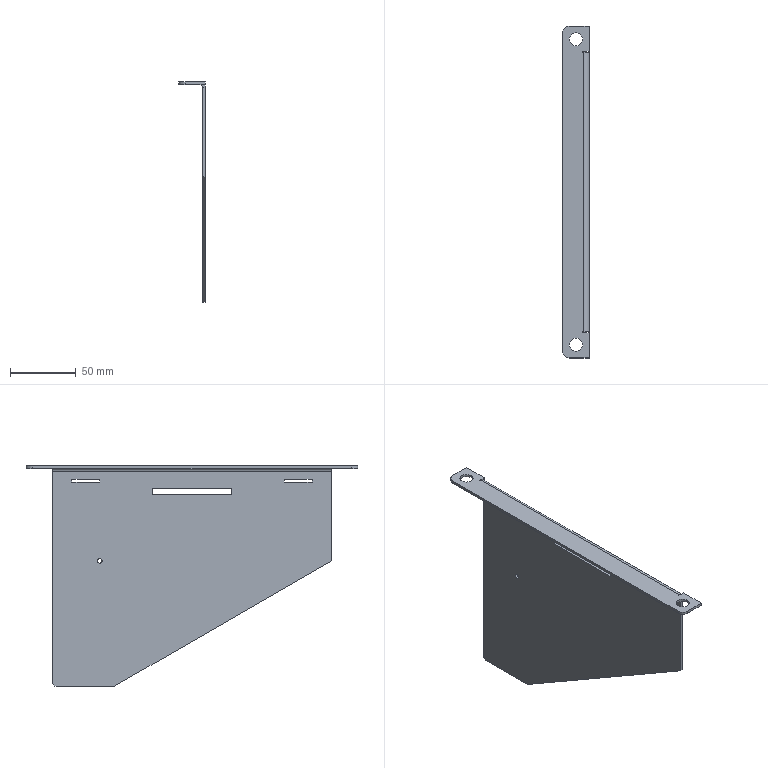Part | STEP file | SYL0380DJ1008_2_7_2_1-1_STEP | 1 solid | 44 faces | box 20 x 252 x 167 mm | volume 62697 mm3 | plane 34 | cylinder 10 | commonest cylinder face diameters 10 x6 3.5 x2 4 x1 8 x1
STEP:
#1=CARTESIAN_POINT('',(10.,-30.,-15.));
#2=VERTEX_POINT('',#1);
#3=CARTESIAN_POINT('',(8.,-30.,-15.));
#4=VERTEX_POINT('',#3);
#5=CARTESIAN_POINT('',(8.,-30.,-15.));
#6=DIRECTION('',(-1.,0.,0.));
#7=VECTOR('',#6,1000.);
#8=LINE('',#5,#7);
#9=EDGE_CURVE('',#2,#4,#8,.T.);
#10=ORIENTED_EDGE('',*,*,#9,.F.);
#11=CARTESIAN_POINT('',(10.,-30.,-20.));
#12=VERTEX_POINT('',#11);
#13=CARTESIAN_POINT('',(10.,-30.,2.));
#14=DIRECTION('',(0.,0.,-1.));
#15=VECTOR('',#14,1000.);
#16=LINE('',#13,#15);
#17=EDGE_CURVE('',#2,#12,#16,.T.);
#18=ORIENTED_EDGE('',*,*,#17,.T.);
#19=CARTESIAN_POINT('',(8.,-30.,-20.));
#20=VERTEX_POINT('',#19);
#21=CARTESIAN_POINT('',(8.,-30.,-20.));
#22=DIRECTION('',(-1.,0.,0.));
#23=VECTOR('',#22,1000.);
#24=LINE('',#21,#23);
#25=EDGE_CURVE('',#12,#20,#24,.T.);
#26=ORIENTED_EDGE('',*,*,#25,.T.);
#27=CARTESIAN_POINT('',(8.,-30.,-15.));
#28=DIRECTION('',(0.,0.,-1.));
#29=VECTOR('',#28,1000.);
#30=LINE('',#27,#29);
#31=EDGE_CURVE('',#4,#20,#30,.T.);
#32=ORIENTED_EDGE('',*,*,#31,.F.);
#33=EDGE_LOOP('',(#10,#18,#26,#32));
#34=FACE_OUTER_BOUND('',#33,.T.);
#35=CARTESIAN_POINT('',(8.,-30.,-15.));
#36=DIRECTION('',(0.,-1.,0.));
#37=DIRECTION('',(0.,0.,-1.));
#38=AXIS2_PLACEMENT_3D('',#35,#36,#37);
#39=PLANE('',#38);
#40=ADVANCED_FACE('',(#34),#39,.F.);
#41=ORIENTED_EDGE('',*,*,#25,.F.);
#42=CARTESIAN_POINT('',(10.,30.,-20.));
#43=VERTEX_POINT('',#42);
#44=CARTESIAN_POINT('',(10.,-66.125,-20.));
#45=DIRECTION('',(0.,1.,0.));
#46=VECTOR('',#45,1000.);
#47=LINE('',#44,#46);
#48=EDGE_CURVE('',#12,#43,#47,.T.);
#49=ORIENTED_EDGE('',*,*,#48,.T.);
#50=CARTESIAN_POINT('',(8.,30.,-20.));
#51=VERTEX_POINT('',#50);
#52=CARTESIAN_POINT('',(8.,30.,-20.));
#53=DIRECTION('',(-1.,0.,0.));
#54=VECTOR('',#53,1000.);
#55=LINE('',#52,#54);
#56=EDGE_CURVE('',#43,#51,#55,.T.);
#57=ORIENTED_EDGE('',*,*,#56,.T.);
#58=CARTESIAN_POINT('',(8.,-30.,-20.));
#59=DIRECTION('',(0.,1.,0.));
#60=VECTOR('',#59,1000.);
#61=LINE('',#58,#60);
#62=EDGE_CURVE('',#20,#51,#61,.T.);
#63=ORIENTED_EDGE('',*,*,#62,.F.);
#64=EDGE_LOOP('',(#41,#49,#57,#63));
#65=FACE_OUTER_BOUND('',#64,.T.);
#66=CARTESIAN_POINT('',(8.,-30.,-20.));
#67=DIRECTION('',(0.,0.,-1.));
#68=DIRECTION('',(0.,1.,0.));
#69=AXIS2_PLACEMENT_3D('',#66,#67,#68);
#70=PLANE('',#69);
#71=ADVANCED_FACE('',(#65),#70,.F.);
#72=ORIENTED_EDGE('',*,*,#56,.F.);
#73=CARTESIAN_POINT('',(10.,30.,-15.));
#74=VERTEX_POINT('',#73);
#75=CARTESIAN_POINT('',(10.,30.,2.));
#76=DIRECTION('',(0.,0.,1.));
#77=VECTOR('',#76,1000.);
#78=LINE('',#75,#77);
#79=EDGE_CURVE('',#43,#74,#78,.T.);
#80=ORIENTED_EDGE('',*,*,#79,.T.);
#81=CARTESIAN_POINT('',(8.,30.,-15.));
#82=VERTEX_POINT('',#81);
#83=CARTESIAN_POINT('',(8.,30.,-15.));
#84=DIRECTION('',(-1.,0.,0.));
#85=VECTOR('',#84,1000.);
#86=LINE('',#83,#85);
#87=EDGE_CURVE('',#74,#82,#86,.T.);
#88=ORIENTED_EDGE('',*,*,#87,.T.);
#89=CARTESIAN_POINT('',(8.,30.,-20.));
#90=DIRECTION('',(0.,0.,1.));
#91=VECTOR('',#90,1000.);
#92=LINE('',#89,#91);
#93=EDGE_CURVE('',#51,#82,#92,.T.);
#94=ORIENTED_EDGE('',*,*,#93,.F.);
#95=EDGE_LOOP('',(#72,#80,#88,#94));
#96=FACE_OUTER_BOUND('',#95,.T.);
#97=CARTESIAN_POINT('',(8.,30.,-20.));
#98=DIRECTION('',(0.,1.,0.));
#99=DIRECTION('',(0.,0.,1.));
#100=AXIS2_PLACEMENT_3D('',#97,#98,#99);
#101=PLANE('',#100);
#102=ADVANCED_FACE('',(#96),#101,.F.);
#103=CARTESIAN_POINT('',(10.,70.,-8.));
#104=VERTEX_POINT('',#103);
#105=CARTESIAN_POINT('',(8.,70.,-8.));
#106=VERTEX_POINT('',#105);
#107=CARTESIAN_POINT('',(8.,70.,-8.));
#108=DIRECTION('',(-1.,0.,0.));
#109=VECTOR('',#108,1000.);
#110=LINE('',#107,#109);
#111=EDGE_CURVE('',#104,#106,#110,.T.);
#112=ORIENTED_EDGE('',*,*,#111,.F.);
#113=CARTESIAN_POINT('',(10.,70.,-10.2));
#114=VERTEX_POINT('',#113);
#115=CARTESIAN_POINT('',(10.,70.,2.));
#116=DIRECTION('',(0.,0.,-1.));
#117=VECTOR('',#116,1000.);
#118=LINE('',#115,#117);
#119=EDGE_CURVE('',#104,#114,#118,.T.);
#120=ORIENTED_EDGE('',*,*,#119,.T.);
#121=CARTESIAN_POINT('',(8.,70.,-10.2));
#122=VERTEX_POINT('',#121);
#123=CARTESIAN_POINT('',(8.,70.,-10.2));
#124=DIRECTION('',(-1.,0.,0.));
#125=VECTOR('',#124,1000.);
#126=LINE('',#123,#125);
#127=EDGE_CURVE('',#114,#122,#126,.T.);
#128=ORIENTED_EDGE('',*,*,#127,.T.);
#129=CARTESIAN_POINT('',(8.,70.,-8.));
#130=DIRECTION('',(0.,0.,-1.));
#131=VECTOR('',#130,1000.);
#132=LINE('',#129,#131);
#133=EDGE_CURVE('',#106,#122,#132,.T.);
#134=ORIENTED_EDGE('',*,*,#133,.F.);
#135=EDGE_LOOP('',(#112,#120,#128,#134));
#136=FACE_OUTER_BOUND('',#135,.T.);
#137=CARTESIAN_POINT('',(8.,70.,-8.));
#138=DIRECTION('',(0.,-1.,0.));
#139=DIRECTION('',(0.,0.,-1.));
#140=AXIS2_PLACEMENT_3D('',#137,#138,#139);
#141=PLANE('',#140);
#142=ADVANCED_FACE('',(#136),#141,.F.);
#143=ORIENTED_EDGE('',*,*,#127,.F.);
#144=CARTESIAN_POINT('',(10.,91.2,-10.2));
#145=VERTEX_POINT('',#144);
#146=CARTESIAN_POINT('',(10.,-66.125,-10.2));
#147=DIRECTION('',(0.,1.,0.));
#148=VECTOR('',#147,1000.);
#149=LINE('',#146,#148);
#150=EDGE_CURVE('',#114,#145,#149,.T.);
#151=ORIENTED_EDGE('',*,*,#150,.T.);
#152=CARTESIAN_POINT('',(8.,91.2,-10.2));
#153=VERTEX_POINT('',#152);
#154=CARTESIAN_POINT('',(8.,91.2,-10.2));
#155=DIRECTION('',(-1.,0.,0.));
#156=VECTOR('',#155,1000.);
#157=LINE('',#154,#156);
#158=EDGE_CURVE('',#145,#153,#157,.T.);
#159=ORIENTED_EDGE('',*,*,#158,.T.);
#160=CARTESIAN_POINT('',(8.,70.,-10.2));
#161=DIRECTION('',(0.,1.,0.));
#162=VECTOR('',#161,1000.);
#163=LINE('',#160,#162);
#164=EDGE_CURVE('',#122,#153,#163,.T.);
#165=ORIENTED_EDGE('',*,*,#164,.F.);
#166=EDGE_LOOP('',(#143,#151,#159,#165));
#167=FACE_OUTER_BOUND('',#166,.T.);
#168=CARTESIAN_POINT('',(8.,70.,-10.2));
#169=DIRECTION('',(0.,0.,-1.));
#170=DIRECTION('',(0.,1.,0.));
#171=AXIS2_PLACEMENT_3D('',#168,#169,#170);
#172=PLANE('',#171);
#173=ADVANCED_FACE('',(#167),#172,.F.);
#174=ORIENTED_EDGE('',*,*,#158,.F.);
#175=CARTESIAN_POINT('',(10.,91.2,-8.));
#176=VERTEX_POINT('',#175);
#177=CARTESIAN_POINT('',(10.,91.2,2.));
#178=DIRECTION('',(0.,0.,1.));
#179=VECTOR('',#178,1000.);
#180=LINE('',#177,#179);
#181=EDGE_CURVE('',#145,#176,#180,.T.);
#182=ORIENTED_EDGE('',*,*,#181,.T.);
#183=CARTESIAN_POINT('',(8.,91.2,-8.));
#184=VERTEX_POINT('',#183);
#185=CARTESIAN_POINT('',(8.,91.2,-8.));
#186=DIRECTION('',(-1.,0.,0.));
#187=VECTOR('',#186,1000.);
#188=LINE('',#185,#187);
#189=EDGE_CURVE('',#176,#184,#188,.T.);
#190=ORIENTED_EDGE('',*,*,#189,.T.);
#191=CARTESIAN_POINT('',(8.,91.2,-10.2));
#192=DIRECTION('',(0.,0.,1.));
#193=VECTOR('',#192,1000.);
#194=LINE('',#191,#193);
#195=EDGE_CURVE('',#153,#184,#194,.T.);
#196=ORIENTED_EDGE('',*,*,#195,.F.);
#197=EDGE_LOOP('',(#174,#182,#190,#196));
#198=FACE_OUTER_BOUND('',#197,.T.);
#199=CARTESIAN_POINT('',(8.,91.2,-10.2));
#200=DIRECTION('',(0.,1.,0.));
#201=DIRECTION('',(0.,0.,1.));
#202=AXIS2_PLACEMENT_3D('',#199,#200,#201);
#203=PLANE('',#202);
#204=ADVANCED_FACE('',(#198),#203,.F.);
#205=CARTESIAN_POINT('',(10.,-91.2,-10.2));
#206=VERTEX_POINT('',#205);
#207=CARTESIAN_POINT('',(8.,-91.2,-10.2));
#208=VERTEX_POINT('',#207);
#209=CARTESIAN_POINT('',(8.,-91.2,-10.2));
#210=DIRECTION('',(-1.,0.,0.));
#211=VECTOR('',#210,1000.);
#212=LINE('',#209,#211);
#213=EDGE_CURVE('',#206,#208,#212,.T.);
#214=ORIENTED_EDGE('',*,*,#213,.F.);
#215=CARTESIAN_POINT('',(10.,-70.,-10.2));
#216=VERTEX_POINT('',#215);
#217=CARTESIAN_POINT('',(10.,-66.125,-10.2));
#218=DIRECTION('',(0.,1.,0.));
#219=VECTOR('',#218,1000.);
#220=LINE('',#217,#219);
#221=EDGE_CURVE('',#206,#216,#220,.T.);
#222=ORIENTED_EDGE('',*,*,#221,.T.);
#223=CARTESIAN_POINT('',(8.,-70.,-10.2));
#224=VERTEX_POINT('',#223);
#225=CARTESIAN_POINT('',(8.,-70.,-10.2));
#226=DIRECTION('',(-1.,0.,0.));
#227=VECTOR('',#226,1000.);
#228=LINE('',#225,#227);
#229=EDGE_CURVE('',#216,#224,#228,.T.);
#230=ORIENTED_EDGE('',*,*,#229,.T.);
#231=CARTESIAN_POINT('',(8.,-91.2,-10.2));
#232=DIRECTION('',(0.,1.,0.));
#233=VECTOR('',#232,1000.);
#234=LINE('',#231,#233);
#235=EDGE_CURVE('',#208,#224,#234,.T.);
#236=ORIENTED_EDGE('',*,*,#235,.F.);
#237=EDGE_LOOP('',(#214,#222,#230,#236));
#238=FACE_OUTER_BOUND('',#237,.T.);
#239=CARTESIAN_POINT('',(8.,-91.2,-10.2));
#240=DIRECTION('',(0.,0.,-1.));
#241=DIRECTION('',(0.,1.,0.));
#242=AXIS2_PLACEMENT_3D('',#239,#240,#241);
#243=PLANE('',#242);
#244=ADVANCED_FACE('',(#238),#243,.F.);
#245=ORIENTED_EDGE('',*,*,#229,.F.);
#246=CARTESIAN_POINT('',(10.,-70.,-8.));
#247=VERTEX_POINT('',#246);
#248=CARTESIAN_POINT('',(10.,-70.,2.));
#249=DIRECTION('',(0.,0.,1.));
#250=VECTOR('',#249,1000.);
#251=LINE('',#248,#250);
#252=EDGE_CURVE('',#216,#247,#251,.T.);
#253=ORIENTED_EDGE('',*,*,#252,.T.);
#254=CARTESIAN_POINT('',(8.,-70.,-8.));
#255=VERTEX_POINT('',#254);
#256=CARTESIAN_POINT('',(8.,-70.,-8.));
#257=DIRECTION('',(-1.,0.,0.));
#258=VECTOR('',#257,1000.);
#259=LINE('',#256,#258);
#260=EDGE_CURVE('',#247,#255,#259,.T.);
#261=ORIENTED_EDGE('',*,*,#260,.T.);
#262=CARTESIAN_POINT('',(8.,-70.,-10.2));
#263=DIRECTION('',(0.,0.,1.));
#264=VECTOR('',#263,1000.);
#265=LINE('',#262,#264);
#266=EDGE_CURVE('',#224,#255,#265,.T.);
#267=ORIENTED_EDGE('',*,*,#266,.F.);
#268=EDGE_LOOP('',(#245,#253,#261,#267));
#269=FACE_OUTER_BOUND('',#268,.T.);
#270=CARTESIAN_POINT('',(8.,-70.,-10.2));
#271=DIRECTION('',(0.,1.,0.));
#272=DIRECTION('',(0.,0.,1.));
#273=AXIS2_PLACEMENT_3D('',#270,#271,#272);
#274=PLANE('',#273);
#275=ADVANCED_FACE('',(#269),#274,.F.);
#276=ORIENTED_EDGE('',*,*,#260,.F.);
#277=CARTESIAN_POINT('',(10.,-91.2,-8.));
#278=VERTEX_POINT('',#277);
#279=CARTESIAN_POINT('',(10.,-66.125,-8.));
#280=DIRECTION('',(0.,-1.,0.));
#281=VECTOR('',#280,1000.);
#282=LINE('',#279,#281);
#283=EDGE_CURVE('',#247,#278,#282,.T.);
#284=ORIENTED_EDGE('',*,*,#283,.T.);
#285=CARTESIAN_POINT('',(8.,-91.2,-8.));
#286=VERTEX_POINT('',#285);
#287=CARTESIAN_POINT('',(8.,-91.2,-8.));
#288=DIRECTION('',(-1.,0.,0.));
#289=VECTOR('',#288,1000.);
#290=LINE('',#287,#289);
#291=EDGE_CURVE('',#278,#286,#290,.T.);
#292=ORIENTED_EDGE('',*,*,#291,.T.);
#293=CARTESIAN_POINT('',(8.,-70.,-8.));
#294=DIRECTION('',(0.,-1.,0.));
#295=VECTOR('',#294,1000.);
#296=LINE('',#293,#295);
#297=EDGE_CURVE('',#255,#286,#296,.T.);
#298=ORIENTED_EDGE('',*,*,#297,.F.);
#299=EDGE_LOOP('',(#276,#284,#292,#298));
#300=FACE_OUTER_BOUND('',#299,.T.);
#301=CARTESIAN_POINT('',(8.,-70.,-8.));
#302=DIRECTION('',(0.,0.,1.));
#303=DIRECTION('',(0.,-1.,0.));
#304=AXIS2_PLACEMENT_3D('',#301,#302,#303);
#305=PLANE('',#304);
#306=ADVANCED_FACE('',(#300),#305,.F.);
#307=CARTESIAN_POINT('',(10.,70.,-71.75));
#308=VERTEX_POINT('',#307);
#309=CARTESIAN_POINT('',(8.,70.,-71.75));
#310=VERTEX_POINT('',#309);
#311=CARTESIAN_POINT('',(8.,70.,-71.75));
#312=DIRECTION('',(-1.,0.,0.));
#313=VECTOR('',#312,1000.);
#314=LINE('',#311,#313);
#315=EDGE_CURVE('',#308,#310,#314,.T.);
#316=ORIENTED_EDGE('',*,*,#315,.F.);
#317=CARTESIAN_POINT('',(10.,70.,-68.25));
#318=VERTEX_POINT('',#317);
#319=CARTESIAN_POINT('',(10.,70.,-70.));
#320=DIRECTION('',(1.,0.,0.));
#321=DIRECTION('',(0.,0.,-1.));
#322=AXIS2_PLACEMENT_3D('',#319,#320,#321);
#323=CIRCLE('',#322,1.75);
#324=EDGE_CURVE('',#308,#318,#323,.T.);
#325=ORIENTED_EDGE('',*,*,#324,.T.);
#326=CARTESIAN_POINT('',(8.,70.,-68.25));
#327=VERTEX_POINT('',#326);
#328=CARTESIAN_POINT('',(8.,70.,-68.25));
#329=DIRECTION('',(-1.,0.,0.));
#330=VECTOR('',#329,1000.);
#331=LINE('',#328,#330);
#332=EDGE_CURVE('',#318,#327,#331,.T.);
#333=ORIENTED_EDGE('',*,*,#332,.T.);
#334=CARTESIAN_POINT('',(8.,70.,-70.));
#335=DIRECTION('',(1.,0.,0.));
#336=DIRECTION('',(0.,0.,-1.));
#337=AXIS2_PLACEMENT_3D('',#334,#335,#336);
#338=CIRCLE('',#337,1.75);
#339=EDGE_CURVE('',#310,#327,#338,.T.);
#340=ORIENTED_EDGE('',*,*,#339,.F.);
#341=EDGE_LOOP('',(#316,#325,#333,#340));
#342=FACE_OUTER_BOUND('',#341,.T.);
#343=CARTESIAN_POINT('',(8.,70.,-70.));
#344=DIRECTION('',(1.,0.,0.));
#345=DIRECTION('',(0.,0.,-1.));
#346=AXIS2_PLACEMENT_3D('',#343,#344,#345);
#347=CYLINDRICAL_SURFACE('',#346,1.75);
#348=ADVANCED_FACE('',(#342),#347,.F.);
#349=CARTESIAN_POINT('',(-5.,116.,2.));
#350=VERTEX_POINT('',#349);
#351=CARTESIAN_POINT('',(-5.,116.,0.));
#352=VERTEX_POINT('',#351);
#353=CARTESIAN_POINT('',(-5.,116.,0.));
#354=DIRECTION('',(0.,0.,-1.));
#355=VECTOR('',#354,1000.);
#356=LINE('',#353,#355);
#357=EDGE_CURVE('',#350,#352,#356,.T.);
#358=ORIENTED_EDGE('',*,*,#357,.F.);
#359=CARTESIAN_POINT('',(5.,116.,2.));
#360=VERTEX_POINT('',#359);
#361=CARTESIAN_POINT('',(0.,116.,2.));
#362=DIRECTION('',(0.,0.,1.));
#363=DIRECTION('',(1.,0.,0.));
#364=AXIS2_PLACEMENT_3D('',#361,#362,#363);
#365=CIRCLE('',#364,5.);
#366=EDGE_CURVE('',#350,#360,#365,.T.);
#367=ORIENTED_EDGE('',*,*,#366,.T.);
#368=CARTESIAN_POINT('',(5.,116.,0.));
#369=VERTEX_POINT('',#368);
#370=CARTESIAN_POINT('',(5.,116.,0.));
#371=DIRECTION('',(0.,0.,-1.));
#372=VECTOR('',#371,1000.);
#373=LINE('',#370,#372);
#374=EDGE_CURVE('',#360,#369,#373,.T.);
#375=ORIENTED_EDGE('',*,*,#374,.T.);
#376=CARTESIAN_POINT('',(0.,116.,0.));
#377=DIRECTION('',(0.,0.,1.));
#378=DIRECTION('',(-1.,0.,0.));
#379=AXIS2_PLACEMENT_3D('',#376,#377,#378);
#380=CIRCLE('',#379,5.);
#381=EDGE_CURVE('',#352,#369,#380,.T.);
#382=ORIENTED_EDGE('',*,*,#381,.F.);
#383=EDGE_LOOP('',(#358,#367,#375,#382));
#384=FACE_OUTER_BOUND('',#383,.T.);
#385=CARTESIAN_POINT('',(0.,116.,0.));
#386=DIRECTION('',(0.,0.,1.));
#387=DIRECTION('',(1.,0.,0.));
#388=AXIS2_PLACEMENT_3D('',#385,#386,#387);
#389=CYLINDRICAL_SURFACE('',#388,5.);
#390=ADVANCED_FACE('',(#384),#389,.F.);
#391=CARTESIAN_POINT('',(-5.,-116.,2.));
#392=VERTEX_POINT('',#391);
#393=CARTESIAN_POINT('',(-5.,-116.,0.));
#394=VERTEX_POINT('',#393);
#395=CARTESIAN_POINT('',(-5.,-116.,0.));
#396=DIRECTION('',(0.,0.,-1.));
#397=VECTOR('',#396,1000.);
#398=LINE('',#395,#397);
#399=EDGE_CURVE('',#392,#394,#398,.T.);
#400=ORIENTED_EDGE('',*,*,#399,.F.);
#401=CARTESIAN_POINT('',(5.,-116.,2.));
#402=VERTEX_POINT('',#401);
#403=CARTESIAN_POINT('',(0.,-116.,2.));
#404=DIRECTION('',(0.,0.,1.));
#405=DIRECTION('',(1.,0.,0.));
#406=AXIS2_PLACEMENT_3D('',#403,#404,#405);
#407=CIRCLE('',#406,5.);
#408=EDGE_CURVE('',#392,#402,#407,.T.);
#409=ORIENTED_EDGE('',*,*,#408,.T.);
#410=CARTESIAN_POINT('',(5.,-116.,0.));
#411=VERTEX_POINT('',#410);
#412=CARTESIAN_POINT('',(5.,-116.,0.));
#413=DIRECTION('',(0.,0.,-1.));
#414=VECTOR('',#413,1000.);
#415=LINE('',#412,#414);
#416=EDGE_CURVE('',#402,#411,#415,.T.);
#417=ORIENTED_EDGE('',*,*,#416,.T.);
#418=CARTESIAN_POINT('',(0.,-116.,0.));
#419=DIRECTION('',(0.,0.,1.));
#420=DIRECTION('',(-1.,0.,0.));
#421=AXIS2_PLACEMENT_3D('',#418,#419,#420);
#422=CIRCLE('',#421,5.);
#423=EDGE_CURVE('',#394,#411,#422,.T.);
#424=ORIENTED_EDGE('',*,*,#423,.F.);
#425=EDGE_LOOP('',(#400,#409,#417,#424));
#426=FACE_OUTER_BOUND('',#425,.T.);
#427=CARTESIAN_POINT('',(0.,-116.,0.));
#428=DIRECTION('',(0.,0.,1.));
#429=DIRECTION('',(1.,0.,0.));
#430=AXIS2_PLACEMENT_3D('',#427,#428,#429);
#431=CYLINDRICAL_SURFACE('',#430,5.);
#432=ADVANCED_FACE('',(#426),#431,.F.);
#433=CARTESIAN_POINT('',(10.,106.,-163.));
#434=VERTEX_POINT('',#433);
#435=CARTESIAN_POINT('',(8.,106.,-163.));
#436=VERTEX_POINT('',#435);
#437=CARTESIAN_POINT('',(8.,106.,-163.));
#438=DIRECTION('',(-1.,0.,0.));
#439=VECTOR('',#438,1000.);
#440=LINE('',#437,#439);
#441=EDGE_CURVE('',#434,#436,#440,.T.);
#442=ORIENTED_EDGE('',*,*,#441,.F.);
#443=CARTESIAN_POINT('',(10.,104.,-165.));
#444=VERTEX_POINT('',#443);
#445=CARTESIAN_POINT('',(10.,106.,-163.));
#446=DIRECTION('',(0.,-0.7071,-0.7071));
#447=VECTOR('',#446,1000.);
#448=LINE('',#445,#447);
#449=EDGE_CURVE('',#434,#444,#448,.T.);
#450=ORIENTED_EDGE('',*,*,#449,.T.);
#451=CARTESIAN_POINT('',(8.,104.,-165.));
#452=VERTEX_POINT('',#451);
#453=CARTESIAN_POINT('',(8.,104.,-165.));
#454=DIRECTION('',(-1.,0.,0.));
#455=VECTOR('',#454,1000.);
#456=LINE('',#453,#455);
#457=EDGE_CURVE('',#444,#452,#456,.T.);
#458=ORIENTED_EDGE('',*,*,#457,.T.);
#459=CARTESIAN_POINT('',(8.,106.,-163.));
#460=DIRECTION('',(0.,-0.7071,-0.7071));
#461=VECTOR('',#460,1000.);
#462=LINE('',#459,#461);
#463=EDGE_CURVE('',#436,#452,#462,.T.);
#464=ORIENTED_EDGE('',*,*,#463,.F.);
#465=EDGE_LOOP('',(#442,#450,#458,#464));
#466=FACE_OUTER_BOUND('',#465,.T.);
#467=CARTESIAN_POINT('',(8.,106.,-163.));
#468=DIRECTION('',(0.,-0.7071,0.7071));
#469=DIRECTION('',(0.,-0.7071,-0.7071));
#470=AXIS2_PLACEMENT_3D('',#467,#468,#469);
#471=PLANE('',#470);
#472=ADVANCED_FACE('',(#466),#471,.F.);
#473=ORIENTED_EDGE('',*,*,#457,.F.);
#474=CARTESIAN_POINT('',(10.,58.545,-165.));
#475=VERTEX_POINT('',#474);
#476=CARTESIAN_POINT('',(10.,-66.125,-165.));
#477=DIRECTION('',(0.,-1.,0.));
#478=VECTOR('',#477,1000.);
#479=LINE('',#476,#478);
#480=EDGE_CURVE('',#444,#475,#479,.T.);
#481=ORIENTED_EDGE('',*,*,#480,.T.);
#482=CARTESIAN_POINT('',(8.,58.545,-165.));
#483=VERTEX_POINT('',#482);
#484=CARTESIAN_POINT('',(8.,58.545,-165.));
#485=DIRECTION('',(-1.,0.,0.));
#486=VECTOR('',#485,1000.);
#487=LINE('',#484,#486);
#488=EDGE_CURVE('',#475,#483,#487,.T.);
#489=ORIENTED_EDGE('',*,*,#488,.T.);
#490=CARTESIAN_POINT('',(8.,104.,-165.));
#491=DIRECTION('',(0.,-1.,0.));
#492=VECTOR('',#491,1000.);
#493=LINE('',#490,#492);
#494=EDGE_CURVE('',#452,#483,#493,.T.);
#495=ORIENTED_EDGE('',*,*,#494,.F.);
#496=EDGE_LOOP('',(#473,#481,#489,#495));
#497=FACE_OUTER_BOUND('',#496,.T.);
#498=CARTESIAN_POINT('',(8.,104.,-165.));
#499=DIRECTION('',(0.,0.,1.));
#500=DIRECTION('',(0.,-1.,0.));
#501=AXIS2_PLACEMENT_3D('',#498,#499,#500);
#502=PLANE('',#501);
#503=ADVANCED_FACE('',(#497),#502,.F.);
#504=ORIENTED_EDGE('',*,*,#488,.F.);
#505=CARTESIAN_POINT('',(10.,-106.,-70.));
#506=VERTEX_POINT('',#505);
#507=CARTESIAN_POINT('',(10.,58.545,-165.));
#508=DIRECTION('',(0.,-0.866,0.5));
#509=VECTOR('',#508,1000.);
#510=LINE('',#507,#509);
#511=EDGE_CURVE('',#475,#506,#510,.T.);
#512=ORIENTED_EDGE('',*,*,#511,.T.);
#513=CARTESIAN_POINT('',(8.,-106.,-70.));
#514=VERTEX_POINT('',#513);
#515=CARTESIAN_POINT('',(8.,-106.,-70.));
#516=DIRECTION('',(-1.,0.,0.));
#517=VECTOR('',#516,1000.);
#518=LINE('',#515,#517);
#519=EDGE_CURVE('',#506,#514,#518,.T.);
#520=ORIENTED_EDGE('',*,*,#519,.T.);
#521=CARTESIAN_POINT('',(8.,58.545,-165.));
#522=DIRECTION('',(0.,-0.866,0.5));
#523=VECTOR('',#522,1000.);
#524=LINE('',#521,#523);
#525=EDGE_CURVE('',#483,#514,#524,.T.);
#526=ORIENTED_EDGE('',*,*,#525,.F.);
#527=EDGE_LOOP('',(#504,#512,#520,#526));
#528=FACE_OUTER_BOUND('',#527,.T.);
#529=CARTESIAN_POINT('',(8.,58.545,-165.));
#530=DIRECTION('',(0.,0.5,0.866));
#531=DIRECTION('',(0.,-0.866,0.5));
#532=AXIS2_PLACEMENT_3D('',#529,#530,#531);
#533=PLANE('',#532);
#534=ADVANCED_FACE('',(#528),#533,.F.);
#535=ORIENTED_EDGE('',*,*,#519,.F.);
#536=CARTESIAN_POINT('',(10.,-106.,-2.));
#537=VERTEX_POINT('',#536);
#538=CARTESIAN_POINT('',(10.,-106.,2.));
#539=DIRECTION('',(0.,0.,1.));
#540=VECTOR('',#539,1000.);
#541=LINE('',#538,#540);
#542=EDGE_CURVE('',#506,#537,#541,.T.);
#543=ORIENTED_EDGE('',*,*,#542,.T.);
#544=CARTESIAN_POINT('',(8.,-106.,-2.));
#545=VERTEX_POINT('',#544);
#546=CARTESIAN_POINT('',(8.,-106.,-2.));
#547=DIRECTION('',(-1.,0.,0.));
#548=VECTOR('',#547,1000.);
#549=LINE('',#546,#548);
#550=EDGE_CURVE('',#537,#545,#549,.T.);
#551=ORIENTED_EDGE('',*,*,#550,.T.);
#552=CARTESIAN_POINT('',(8.,-106.,-70.));
#553=DIRECTION('',(0.,0.,1.));
#554=VECTOR('',#553,1000.);
#555=LINE('',#552,#554);
#556=EDGE_CURVE('',#514,#545,#555,.T.);
#557=ORIENTED_EDGE('',*,*,#556,.F.);
#558=EDGE_LOOP('',(#535,#543,#551,#557));
#559=FACE_OUTER_BOUND('',#558,.T.);
#560=CARTESIAN_POINT('',(8.,-106.,-70.));
#561=DIRECTION('',(0.,1.,0.));
#562=DIRECTION('',(0.,0.,1.));
#563=AXIS2_PLACEMENT_3D('',#560,#561,#562);
#564=PLANE('',#563);
#565=ADVANCED_FACE('',(#559),#564,.F.);
#566=ORIENTED_EDGE('',*,*,#550,.F.);
#567=CARTESIAN_POINT('',(6.,-106.,2.));
#568=VERTEX_POINT('',#567);
#569=CARTESIAN_POINT('',(6.,-106.,-2.));
#570=DIRECTION('',(0.,1.,0.));
#571=DIRECTION('',(0.,0.,-1.));
#572=AXIS2_PLACEMENT_3D('',#569,#570,#571);
#573=CIRCLE('',#572,4.);
#574=EDGE_CURVE('',#568,#537,#573,.T.);
#575=ORIENTED_EDGE('',*,*,#574,.F.);
#576=CARTESIAN_POINT('',(6.,-106.,0.));
#577=VERTEX_POINT('',#576);
#578=CARTESIAN_POINT('',(6.,-106.,0.));
#579=DIRECTION('',(0.,0.,-1.));
#580=VECTOR('',#579,1000.);
#581=LINE('',#578,#580);
#582=EDGE_CURVE('',#568,#577,#581,.T.);
#583=ORIENTED_EDGE('',*,*,#582,.T.);
#584=CARTESIAN_POINT('',(6.,-106.,-2.));
#585=DIRECTION('',(0.,1.,0.));
#586=DIRECTION('',(0.,0.,1.));
#587=AXIS2_PLACEMENT_3D('',#584,#585,#586);
#588=CIRCLE('',#587,2.);
#589=EDGE_CURVE('',#577,#545,#588,.T.);
#590=ORIENTED_EDGE('',*,*,#589,.T.);
#591=EDGE_LOOP('',(#566,#575,#583,#590));
#592=FACE_OUTER_BOUND('',#591,.T.);
#593=CARTESIAN_POINT('',(6.,-106.,-2.));
#594=DIRECTION('',(0.,-1.,0.));
#595=DIRECTION('',(0.,0.,-1.));
#596=AXIS2_PLACEMENT_3D('',#593,#594,#595);
#597=PLANE('',#596);
#598=ADVANCED_FACE('',(#592),#597,.T.);
#599=ORIENTED_EDGE('',*,*,#582,.F.);
#600=CARTESIAN_POINT('',(5.,-106.,2.));
#601=VERTEX_POINT('',#600);
#602=CARTESIAN_POINT('',(0.,-106.,2.));
#603=DIRECTION('',(-1.,0.,0.));
#604=VECTOR('',#603,1000.);
#605=LINE('',#602,#604);
#606=EDGE_CURVE('',#568,#601,#605,.T.);
#607=ORIENTED_EDGE('',*,*,#606,.T.);
#608=CARTESIAN_POINT('',(5.,-106.,0.));
#609=VERTEX_POINT('',#608);
#610=CARTESIAN_POINT('',(5.,-106.,0.));
#611=DIRECTION('',(0.,0.,-1.));
#612=VECTOR('',#611,1000.);
#613=LINE('',#610,#612);
#614=EDGE_CURVE('',#601,#609,#613,.T.);
#615=ORIENTED_EDGE('',*,*,#614,.T.);
#616=CARTESIAN_POINT('',(0.,-106.,0.));
#617=DIRECTION('',(-1.,0.,0.));
#618=VECTOR('',#617,1000.);
#619=LINE('',#616,#618);
#620=EDGE_CURVE('',#577,#609,#619,.T.);
#621=ORIENTED_EDGE('',*,*,#620,.F.);
#622=EDGE_LOOP('',(#599,#607,#615,#621));
#623=FACE_OUTER_BOUND('',#622,.T.);
#624=CARTESIAN_POINT('',(0.,-106.,0.));
#625=DIRECTION('',(0.,1.,0.));
#626=DIRECTION('',(-1.,0.,0.));
#627=AXIS2_PLACEMENT_3D('',#624,#625,#626);
#628=PLANE('',#627);
#629=ADVANCED_FACE('',(#623),#628,.F.);
#630=ORIENTED_EDGE('',*,*,#614,.F.);
#631=CARTESIAN_POINT('',(5.,-107.,2.));
#632=VERTEX_POINT('',#631);
#633=CARTESIAN_POINT('',(5.,0.,2.));
#634=DIRECTION('',(0.,-1.,0.));
#635=VECTOR('',#634,1000.);
#636=LINE('',#633,#635);
#637=EDGE_CURVE('',#601,#632,#636,.T.);
#638=ORIENTED_EDGE('',*,*,#637,.T.);
#639=CARTESIAN_POINT('',(5.,-107.,0.));
#640=VERTEX_POINT('',#639);
#641=CARTESIAN_POINT('',(5.,-107.,0.));
#642=DIRECTION('',(0.,0.,-1.));
#643=VECTOR('',#642,1000.);
#644=LINE('',#641,#643);
#645=EDGE_CURVE('',#632,#640,#644,.T.);
#646=ORIENTED_EDGE('',*,*,#645,.T.);
#647=CARTESIAN_POINT('',(5.,0.,0.));
#648=DIRECTION('',(0.,-1.,0.));
#649=VECTOR('',#648,1000.);
#650=LINE('',#647,#649);
#651=EDGE_CURVE('',#609,#640,#650,.T.);
#652=ORIENTED_EDGE('',*,*,#651,.F.);
#653=EDGE_LOOP('',(#630,#638,#646,#652));
#654=FACE_OUTER_BOUND('',#653,.T.);
#655=CARTESIAN_POINT('',(5.,0.,0.));
#656=DIRECTION('',(-1.,0.,0.));
#657=DIRECTION('',(0.,-1.,0.));
#658=AXIS2_PLACEMENT_3D('',#655,#656,#657);
#659=PLANE('',#658);
#660=ADVANCED_FACE('',(#654),#659,.F.);
#661=ORIENTED_EDGE('',*,*,#645,.F.);
#662=CARTESIAN_POINT('',(10.,-107.,2.));
#663=VERTEX_POINT('',#662);
#664=CARTESIAN_POINT('',(0.,-107.,2.));
#665=DIRECTION('',(1.,0.,0.));
#666=VECTOR('',#665,1000.);
#667=LINE('',#664,#666);
#668=EDGE_CURVE('',#632,#663,#667,.T.);
#669=ORIENTED_EDGE('',*,*,#668,.T.);
#670=CARTESIAN_POINT('',(10.,-107.,0.));
#671=VERTEX_POINT('',#670);
#672=CARTESIAN_POINT('',(10.,-107.,0.));
#673=DIRECTION('',(0.,0.,-1.));
#674=VECTOR('',#673,1000.);
#675=LINE('',#672,#674);
#676=EDGE_CURVE('',#663,#671,#675,.T.);
#677=ORIENTED_EDGE('',*,*,#676,.T.);
#678=CARTESIAN_POINT('',(0.,-107.,0.));
#679=DIRECTION('',(1.,0.,0.));
#680=VECTOR('',#679,1000.);
#681=LINE('',#678,#680);
#682=EDGE_CURVE('',#640,#671,#681,.T.);
#683=ORIENTED_EDGE('',*,*,#682,.F.);
#684=EDGE_LOOP('',(#661,#669,#677,#683));
#685=FACE_OUTER_BOUND('',#684,.T.);
#686=CARTESIAN_POINT('',(0.,-107.,0.));
#687=DIRECTION('',(0.,-1.,0.));
#688=DIRECTION('',(1.,0.,0.));
#689=AXIS2_PLACEMENT_3D('',#686,#687,#688);
#690=PLANE('',#689);
#691=ADVANCED_FACE('',(#685),#690,.F.);
#692=ORIENTED_EDGE('',*,*,#676,.F.);
#693=CARTESIAN_POINT('',(10.,-126.,2.));
#694=VERTEX_POINT('',#693);
#695=CARTESIAN_POINT('',(10.,0.,2.));
#696=DIRECTION('',(0.,1.,0.));
#697=VECTOR('',#696,1000.);
#698=LINE('',#695,#697);
#699=EDGE_CURVE('',#694,#663,#698,.T.);
#700=ORIENTED_EDGE('',*,*,#699,.F.);
#701=CARTESIAN_POINT('',(10.,-126.,0.));
#702=VERTEX_POINT('',#701);
#703=CARTESIAN_POINT('',(10.,-126.,0.));
#704=DIRECTION('',(0.,0.,-1.));
#705=VECTOR('',#704,1000.);
#706=LINE('',#703,#705);
#707=EDGE_CURVE('',#694,#702,#706,.T.);
#708=ORIENTED_EDGE('',*,*,#707,.T.);
#709=CARTESIAN_POINT('',(10.,-126.,0.));
#710=DIRECTION('',(0.,1.,0.));
#711=VECTOR('',#710,1000.);
#712=LINE('',#709,#711);
#713=EDGE_CURVE('',#702,#671,#712,.T.);
#714=ORIENTED_EDGE('',*,*,#713,.T.);
#715=EDGE_LOOP('',(#692,#700,#708,#714));
#716=FACE_OUTER_BOUND('',#715,.T.);
#717=CARTESIAN_POINT('',(10.,-126.,0.));
#718=DIRECTION('',(1.,0.,0.));
#719=DIRECTION('',(0.,1.,0.));
#720=AXIS2_PLACEMENT_3D('',#717,#718,#719);
#721=PLANE('',#720);
#722=ADVANCED_FACE('',(#716),#721,.T.);
#723=ORIENTED_EDGE('',*,*,#707,.F.);
#724=CARTESIAN_POINT('',(-5.,-126.,2.));
#725=VERTEX_POINT('',#724);
#726=CARTESIAN_POINT('',(0.,-126.,2.));
#727=DIRECTION('',(1.,0.,0.));
#728=VECTOR('',#727,1000.);
#729=LINE('',#726,#728);
#730=EDGE_CURVE('',#725,#694,#729,.T.);
#731=ORIENTED_EDGE('',*,*,#730,.F.);
#732=CARTESIAN_POINT('',(-5.,-126.,0.));
#733=VERTEX_POINT('',#732);
#734=CARTESIAN_POINT('',(-5.,-126.,0.));
#735=DIRECTION('',(0.,0.,-1.));
#736=VECTOR('',#735,1000.);
#737=LINE('',#734,#736);
#738=EDGE_CURVE('',#725,#733,#737,.T.);
#739=ORIENTED_EDGE('',*,*,#738,.T.);
#740=CARTESIAN_POINT('',(-5.,-126.,0.));
#741=DIRECTION('',(1.,0.,0.));
#742=VECTOR('',#741,1000.);
#743=LINE('',#740,#742);
#744=EDGE_CURVE('',#733,#702,#743,.T.);
#745=ORIENTED_EDGE('',*,*,#744,.T.);
#746=EDGE_LOOP('',(#723,#731,#739,#745));
#747=FACE_OUTER_BOUND('',#746,.T.);
#748=CARTESIAN_POINT('',(-5.,-126.,0.));
#749=DIRECTION('',(0.,-1.,0.));
#750=DIRECTION('',(1.,0.,0.));
#751=AXIS2_PLACEMENT_3D('',#748,#749,#750);
#752=PLANE('',#751);
#753=ADVANCED_FACE('',(#747),#752,.T.);
#754=ORIENTED_EDGE('',*,*,#738,.F.);
#755=CARTESIAN_POINT('',(-10.,-121.,2.));
#756=VERTEX_POINT('',#755);
#757=CARTESIAN_POINT('',(-5.,-121.,2.));
#758=DIRECTION('',(0.,0.,-1.));
#759=DIRECTION('',(-1.,0.,0.));
#760=AXIS2_PLACEMENT_3D('',#757,#758,#759);
#761=CIRCLE('',#760,5.);
#762=EDGE_CURVE('',#725,#756,#761,.T.);
#763=ORIENTED_EDGE('',*,*,#762,.T.);
#764=CARTESIAN_POINT('',(-10.,-121.,0.));
#765=VERTEX_POINT('',#764);
#766=CARTESIAN_POINT('',(-10.,-121.,0.));
#767=DIRECTION('',(0.,0.,-1.));
#768=VECTOR('',#767,1000.);
#769=LINE('',#766,#768);
#770=EDGE_CURVE('',#756,#765,#769,.T.);
#771=ORIENTED_EDGE('',*,*,#770,.T.);
#772=CARTESIAN_POINT('',(-5.,-121.,0.));
#773=DIRECTION('',(0.,0.,-1.));
#774=DIRECTION('',(0.,-1.,0.));
#775=AXIS2_PLACEMENT_3D('',#772,#773,#774);
#776=CIRCLE('',#775,5.);
#777=EDGE_CURVE('',#733,#765,#776,.T.);
#778=ORIENTED_EDGE('',*,*,#777,.F.);
#779=EDGE_LOOP('',(#754,#763,#771,#778));
#780=FACE_OUTER_BOUND('',#779,.T.);
#781=CARTESIAN_POINT('',(-5.,-121.,0.));
#782=DIRECTION('',(0.,0.,1.));
#783=DIRECTION('',(1.,0.,0.));
#784=AXIS2_PLACEMENT_3D('',#781,#782,#783);
#785=CYLINDRICAL_SURFACE('',#784,5.);
#786=ADVANCED_FACE('',(#780),#785,.T.);
#787=ORIENTED_EDGE('',*,*,#770,.F.);
#788=CARTESIAN_POINT('',(-10.,121.,2.));
#789=VERTEX_POINT('',#788);
#790=CARTESIAN_POINT('',(-10.,0.,2.));
#791=DIRECTION('',(0.,-1.,0.));
#792=VECTOR('',#791,1000.);
#793=LINE('',#790,#792);
#794=EDGE_CURVE('',#789,#756,#793,.T.);
#795=ORIENTED_EDGE('',*,*,#794,.F.);
#796=CARTESIAN_POINT('',(-10.,121.,0.));
#797=VERTEX_POINT('',#796);
#798=CARTESIAN_POINT('',(-10.,121.,0.));
#799=DIRECTION('',(0.,0.,-1.));
#800=VECTOR('',#799,1000.);
#801=LINE('',#798,#800);
#802=EDGE_CURVE('',#789,#797,#801,.T.);
#803=ORIENTED_EDGE('',*,*,#802,.T.);
#804=CARTESIAN_POINT('',(-10.,121.,0.));
#805=DIRECTION('',(0.,-1.,0.));
#806=VECTOR('',#805,1000.);
#807=LINE('',#804,#806);
#808=EDGE_CURVE('',#797,#765,#807,.T.);
#809=ORIENTED_EDGE('',*,*,#808,.T.);
#810=EDGE_LOOP('',(#787,#795,#803,#809));
#811=FACE_OUTER_BOUND('',#810,.T.);
#812=CARTESIAN_POINT('',(-10.,121.,0.));
#813=DIRECTION('',(-1.,0.,0.));
#814=DIRECTION('',(0.,-1.,0.));
#815=AXIS2_PLACEMENT_3D('',#812,#813,#814);
#816=PLANE('',#815);
#817=ADVANCED_FACE('',(#811),#816,.T.);
#818=ORIENTED_EDGE('',*,*,#802,.F.);
#819=CARTESIAN_POINT('',(-5.,126.,2.));
#820=VERTEX_POINT('',#819);
#821=CARTESIAN_POINT('',(-5.,121.,2.));
#822=DIRECTION('',(0.,0.,-1.));
#823=DIRECTION('',(-1.,0.,0.));
#824=AXIS2_PLACEMENT_3D('',#821,#822,#823);
#825=CIRCLE('',#824,5.);
#826=EDGE_CURVE('',#789,#820,#825,.T.);
#827=ORIENTED_EDGE('',*,*,#826,.T.);
#828=CARTESIAN_POINT('',(-5.,126.,0.));
#829=VERTEX_POINT('',#828);
#830=CARTESIAN_POINT('',(-5.,126.,0.));
#831=DIRECTION('',(0.,0.,-1.));
#832=VECTOR('',#831,1000.);
#833=LINE('',#830,#832);
#834=EDGE_CURVE('',#820,#829,#833,.T.);
#835=ORIENTED_EDGE('',*,*,#834,.T.);
#836=CARTESIAN_POINT('',(-5.,121.,0.));
#837=DIRECTION('',(0.,0.,-1.));
#838=DIRECTION('',(-1.,0.,0.));
#839=AXIS2_PLACEMENT_3D('',#836,#837,#838);
#840=CIRCLE('',#839,5.);
#841=EDGE_CURVE('',#797,#829,#840,.T.);
#842=ORIENTED_EDGE('',*,*,#841,.F.);
#843=EDGE_LOOP('',(#818,#827,#835,#842));
#844=FACE_OUTER_BOUND('',#843,.T.);
#845=CARTESIAN_POINT('',(-5.,121.,0.));
#846=DIRECTION('',(0.,0.,1.));
#847=DIRECTION('',(1.,0.,0.));
#848=AXIS2_PLACEMENT_3D('',#845,#846,#847);
#849=CYLINDRICAL_SURFACE('',#848,5.);
#850=ADVANCED_FACE('',(#844),#849,.T.);
#851=ORIENTED_EDGE('',*,*,#834,.F.);
#852=CARTESIAN_POINT('',(10.,126.,2.));
#853=VERTEX_POINT('',#852);
#854=CARTESIAN_POINT('',(0.,126.,2.));
#855=DIRECTION('',(-1.,0.,0.));
#856=VECTOR('',#855,1000.);
#857=LINE('',#854,#856);
#858=EDGE_CURVE('',#853,#820,#857,.T.);
#859=ORIENTED_EDGE('',*,*,#858,.F.);
#860=CARTESIAN_POINT('',(10.,126.,0.));
#861=VERTEX_POINT('',#860);
#862=CARTESIAN_POINT('',(10.,126.,0.));
#863=DIRECTION('',(0.,0.,-1.));
#864=VECTOR('',#863,1000.);
#865=LINE('',#862,#864);
#866=EDGE_CURVE('',#853,#861,#865,.T.);
#867=ORIENTED_EDGE('',*,*,#866,.T.);
#868=CARTESIAN_POINT('',(10.,126.,0.));
#869=DIRECTION('',(-1.,0.,0.));
#870=VECTOR('',#869,1000.);
#871=LINE('',#868,#870);
#872=EDGE_CURVE('',#861,#829,#871,.T.);
#873=ORIENTED_EDGE('',*,*,#872,.T.);
#874=EDGE_LOOP('',(#851,#859,#867,#873));
#875=FACE_OUTER_BOUND('',#874,.T.);
#876=CARTESIAN_POINT('',(10.,126.,0.));
#877=DIRECTION('',(0.,1.,0.));
#878=DIRECTION('',(-1.,0.,0.));
#879=AXIS2_PLACEMENT_3D('',#876,#877,#878);
#880=PLANE('',#879);
#881=ADVANCED_FACE('',(#875),#880,.T.);
#882=ORIENTED_EDGE('',*,*,#866,.F.);
#883=CARTESIAN_POINT('',(10.,107.,2.));
#884=VERTEX_POINT('',#883);
#885=CARTESIAN_POINT('',(10.,0.,2.));
#886=DIRECTION('',(0.,1.,0.));
#887=VECTOR('',#886,1000.);
#888=LINE('',#885,#887);
#889=EDGE_CURVE('',#884,#853,#888,.T.);
#890=ORIENTED_EDGE('',*,*,#889,.F.);
#891=CARTESIAN_POINT('',(10.,107.,0.));
#892=VERTEX_POINT('',#891);
#893=CARTESIAN_POINT('',(10.,107.,0.));
#894=DIRECTION('',(0.,0.,-1.));
#895=VECTOR('',#894,1000.);
#896=LINE('',#893,#895);
#897=EDGE_CURVE('',#884,#892,#896,.T.);
#898=ORIENTED_EDGE('',*,*,#897,.T.);
#899=CARTESIAN_POINT('',(10.,106.,0.));
#900=DIRECTION('',(0.,1.,0.));
#901=VECTOR('',#900,1000.);
#902=LINE('',#899,#901);
#903=EDGE_CURVE('',#892,#861,#902,.T.);
#904=ORIENTED_EDGE('',*,*,#903,.T.);
#905=EDGE_LOOP('',(#882,#890,#898,#904));
#906=FACE_OUTER_BOUND('',#905,.T.);
#907=CARTESIAN_POINT('',(10.,106.,0.));
#908=DIRECTION('',(1.,0.,0.));
#909=DIRECTION('',(0.,1.,0.));
#910=AXIS2_PLACEMENT_3D('',#907,#908,#909);
#911=PLANE('',#910);
#912=ADVANCED_FACE('',(#906),#911,.T.);
#913=ORIENTED_EDGE('',*,*,#897,.F.);
#914=CARTESIAN_POINT('',(5.,107.,2.));
#915=VERTEX_POINT('',#914);
#916=CARTESIAN_POINT('',(0.,107.,2.));
#917=DIRECTION('',(-1.,0.,0.));
#918=VECTOR('',#917,1000.);
#919=LINE('',#916,#918);
#920=EDGE_CURVE('',#884,#915,#919,.T.);
#921=ORIENTED_EDGE('',*,*,#920,.T.);
#922=CARTESIAN_POINT('',(5.,107.,0.));
#923=VERTEX_POINT('',#922);
#924=CARTESIAN_POINT('',(5.,107.,0.));
#925=DIRECTION('',(0.,0.,-1.));
#926=VECTOR('',#925,1000.);
#927=LINE('',#924,#926);
#928=EDGE_CURVE('',#915,#923,#927,.T.);
#929=ORIENTED_EDGE('',*,*,#928,.T.);
#930=CARTESIAN_POINT('',(0.,107.,0.));
#931=DIRECTION('',(-1.,0.,0.));
#932=VECTOR('',#931,1000.);
#933=LINE('',#930,#932);
#934=EDGE_CURVE('',#892,#923,#933,.T.);
#935=ORIENTED_EDGE('',*,*,#934,.F.);
#936=EDGE_LOOP('',(#913,#921,#929,#935));
#937=FACE_OUTER_BOUND('',#936,.T.);
#938=CARTESIAN_POINT('',(0.,107.,0.));
#939=DIRECTION('',(0.,1.,0.));
#940=DIRECTION('',(-1.,0.,0.));
#941=AXIS2_PLACEMENT_3D('',#938,#939,#940);
#942=PLANE('',#941);
#943=ADVANCED_FACE('',(#937),#942,.F.);
#944=ORIENTED_EDGE('',*,*,#928,.F.);
#945=CARTESIAN_POINT('',(5.,106.,2.));
#946=VERTEX_POINT('',#945);
#947=CARTESIAN_POINT('',(5.,0.,2.));
#948=DIRECTION('',(0.,-1.,0.));
#949=VECTOR('',#948,1000.);
#950=LINE('',#947,#949);
#951=EDGE_CURVE('',#915,#946,#950,.T.);
#952=ORIENTED_EDGE('',*,*,#951,.T.);
#953=CARTESIAN_POINT('',(5.,106.,0.));
#954=VERTEX_POINT('',#953);
#955=CARTESIAN_POINT('',(5.,106.,0.));
#956=DIRECTION('',(0.,0.,-1.));
#957=VECTOR('',#956,1000.);
#958=LINE('',#955,#957);
#959=EDGE_CURVE('',#946,#954,#958,.T.);
#960=ORIENTED_EDGE('',*,*,#959,.T.);
#961=CARTESIAN_POINT('',(5.,0.,0.));
#962=DIRECTION('',(0.,-1.,0.));
#963=VECTOR('',#962,1000.);
#964=LINE('',#961,#963);
#965=EDGE_CURVE('',#923,#954,#964,.T.);
#966=ORIENTED_EDGE('',*,*,#965,.F.);
#967=EDGE_LOOP('',(#944,#952,#960,#966));
#968=FACE_OUTER_BOUND('',#967,.T.);
#969=CARTESIAN_POINT('',(5.,0.,0.));
#970=DIRECTION('',(-1.,0.,0.));
#971=DIRECTION('',(0.,-1.,0.));
#972=AXIS2_PLACEMENT_3D('',#969,#970,#971);
#973=PLANE('',#972);
#974=ADVANCED_FACE('',(#968),#973,.F.);
#975=ORIENTED_EDGE('',*,*,#959,.F.);
#976=CARTESIAN_POINT('',(6.,106.,2.));
#977=VERTEX_POINT('',#976);
#978=CARTESIAN_POINT('',(0.,106.,2.));
#979=DIRECTION('',(1.,0.,0.));
#980=VECTOR('',#979,1000.);
#981=LINE('',#978,#980);
#982=EDGE_CURVE('',#946,#977,#981,.T.);
#983=ORIENTED_EDGE('',*,*,#982,.T.);
#984=CARTESIAN_POINT('',(6.,106.,0.));
#985=VERTEX_POINT('',#984);
#986=CARTESIAN_POINT('',(6.,106.,0.));
#987=DIRECTION('',(0.,0.,-1.));
#988=VECTOR('',#987,1000.);
#989=LINE('',#986,#988);
#990=EDGE_CURVE('',#977,#985,#989,.T.);
#991=ORIENTED_EDGE('',*,*,#990,.T.);
#992=CARTESIAN_POINT('',(0.,106.,0.));
#993=DIRECTION('',(1.,0.,0.));
#994=VECTOR('',#993,1000.);
#995=LINE('',#992,#994);
#996=EDGE_CURVE('',#954,#985,#995,.T.);
#997=ORIENTED_EDGE('',*,*,#996,.F.);
#998=EDGE_LOOP('',(#975,#983,#991,#997));
#999=FACE_OUTER_BOUND('',#998,.T.);
#1000=CARTESIAN_POINT('',(0.,106.,0.));
#1001=DIRECTION('',(0.,-1.,0.));
#1002=DIRECTION('',(1.,0.,0.));
#1003=AXIS2_PLACEMENT_3D('',#1000,#1001,#1002);
#1004=PLANE('',#1003);
#1005=ADVANCED_FACE('',(#999),#1004,.F.);
#1006=ORIENTED_EDGE('',*,*,#990,.F.);
#1007=CARTESIAN_POINT('',(10.,106.,-2.));
#1008=VERTEX_POINT('',#1007);
#1009=CARTESIAN_POINT('',(6.,106.,-2.));
#1010=DIRECTION('',(0.,-1.,0.));
#1011=DIRECTION('',(0.,0.,-1.));
#1012=AXIS2_PLACEMENT_3D('',#1009,#1010,#1011);
#1013=CIRCLE('',#1012,4.);
#1014=EDGE_CURVE('',#1008,#977,#1013,.T.);
#1015=ORIENTED_EDGE('',*,*,#1014,.F.);
#1016=CARTESIAN_POINT('',(8.,106.,-2.));
#1017=VERTEX_POINT('',#1016);
#1018=CARTESIAN_POINT('',(8.,106.,-2.));
#1019=DIRECTION('',(-1.,0.,0.));
#1020=VECTOR('',#1019,1000.);
#1021=LINE('',#1018,#1020);
#1022=EDGE_CURVE('',#1008,#1017,#1021,.T.);
#1023=ORIENTED_EDGE('',*,*,#1022,.T.);
#1024=CARTESIAN_POINT('',(6.,106.,-2.));
#1025=DIRECTION('',(0.,-1.,0.));
#1026=DIRECTION('',(1.,0.,0.));
#1027=AXIS2_PLACEMENT_3D('',#1024,#1025,#1026);
#1028=CIRCLE('',#1027,2.);
#1029=EDGE_CURVE('',#1017,#985,#1028,.T.);
#1030=ORIENTED_EDGE('',*,*,#1029,.T.);
#1031=EDGE_LOOP('',(#1006,#1015,#1023,#1030));
#1032=FACE_OUTER_BOUND('',#1031,.T.);
#1033=CARTESIAN_POINT('',(6.,106.,-2.));
#1034=DIRECTION('',(0.,1.,0.));
#1035=DIRECTION('',(0.,0.,1.));
#1036=AXIS2_PLACEMENT_3D('',#1033,#1034,#1035);
#1037=PLANE('',#1036);
#1038=ADVANCED_FACE('',(#1032),#1037,.T.);
#1039=CARTESIAN_POINT('',(10.,70.,-70.));
#1040=DIRECTION('',(1.,0.,0.));
#1041=DIRECTION('',(0.,0.,-1.));
#1042=AXIS2_PLACEMENT_3D('',#1039,#1040,#1041);
#1043=CIRCLE('',#1042,1.75);
#1044=EDGE_CURVE('',#318,#308,#1043,.T.);
#1045=ORIENTED_EDGE('',*,*,#1044,.T.);
#1046=ORIENTED_EDGE('',*,*,#315,.T.);
#1047=CARTESIAN_POINT('',(8.,70.,-70.));
#1048=DIRECTION('',(1.,0.,0.));
#1049=DIRECTION('',(0.,0.,1.));
#1050=AXIS2_PLACEMENT_3D('',#1047,#1048,#1049);
#1051=CIRCLE('',#1050,1.75);
#1052=EDGE_CURVE('',#327,#310,#1051,.T.);
#1053=ORIENTED_EDGE('',*,*,#1052,.F.);
#1054=ORIENTED_EDGE('',*,*,#332,.F.);
#1055=EDGE_LOOP('',(#1045,#1046,#1053,#1054));
#1056=FACE_OUTER_BOUND('',#1055,.T.);
#1057=CARTESIAN_POINT('',(8.,70.,-70.));
#1058=DIRECTION('',(1.,0.,0.));
#1059=DIRECTION('',(0.,0.,-1.));
#1060=AXIS2_PLACEMENT_3D('',#1057,#1058,#1059);
#1061=CYLINDRICAL_SURFACE('',#1060,1.75);
#1062=ADVANCED_FACE('',(#1056),#1061,.F.);
#1063=CARTESIAN_POINT('',(10.,-91.2,2.));
#1064=DIRECTION('',(0.,0.,-1.));
#1065=VECTOR('',#1064,1000.);
#1066=LINE('',#1063,#1065);
#1067=EDGE_CURVE('',#278,#206,#1066,.T.);
#1068=ORIENTED_EDGE('',*,*,#1067,.T.);
#1069=ORIENTED_EDGE('',*,*,#213,.T.);
#1070=CARTESIAN_POINT('',(8.,-91.2,-8.));
#1071=DIRECTION('',(0.,0.,-1.));
#1072=VECTOR('',#1071,1000.);
#1073=LINE('',#1070,#1072);
#1074=EDGE_CURVE('',#286,#208,#1073,.T.);
#1075=ORIENTED_EDGE('',*,*,#1074,.F.);
#1076=ORIENTED_EDGE('',*,*,#291,.F.);
#1077=EDGE_LOOP('',(#1068,#1069,#1075,#1076));
#1078=FACE_OUTER_BOUND('',#1077,.T.);
#1079=CARTESIAN_POINT('',(8.,-91.2,-8.));
#1080=DIRECTION('',(0.,-1.,0.));
#1081=DIRECTION('',(0.,0.,-1.));
#1082=AXIS2_PLACEMENT_3D('',#1079,#1080,#1081);
#1083=PLANE('',#1082);
#1084=ADVANCED_FACE('',(#1078),#1083,.F.);
#1085=CARTESIAN_POINT('',(10.,-66.125,-8.));
#1086=DIRECTION('',(0.,-1.,0.));
#1087=VECTOR('',#1086,1000.);
#1088=LINE('',#1085,#1087);
#1089=EDGE_CURVE('',#176,#104,#1088,.T.);
#1090=ORIENTED_EDGE('',*,*,#1089,.T.);
#1091=ORIENTED_EDGE('',*,*,#111,.T.);
#1092=CARTESIAN_POINT('',(8.,91.2,-8.));
#1093=DIRECTION('',(0.,-1.,0.));
#1094=VECTOR('',#1093,1000.);
#1095=LINE('',#1092,#1094);
#1096=EDGE_CURVE('',#184,#106,#1095,.T.);
#1097=ORIENTED_EDGE('',*,*,#1096,.F.);
#1098=ORIENTED_EDGE('',*,*,#189,.F.);
#1099=EDGE_LOOP('',(#1090,#1091,#1097,#1098));
#1100=FACE_OUTER_BOUND('',#1099,.T.);
#1101=CARTESIAN_POINT('',(8.,91.2,-8.));
#1102=DIRECTION('',(0.,0.,1.));
#1103=DIRECTION('',(0.,-1.,0.));
#1104=AXIS2_PLACEMENT_3D('',#1101,#1102,#1103);
#1105=PLANE('',#1104);
#1106=ADVANCED_FACE('',(#1100),#1105,.F.);
#1107=CARTESIAN_POINT('',(10.,-66.125,-15.));
#1108=DIRECTION('',(0.,-1.,0.));
#1109=VECTOR('',#1108,1000.);
#1110=LINE('',#1107,#1109);
#1111=EDGE_CURVE('',#74,#2,#1110,.T.);
#1112=ORIENTED_EDGE('',*,*,#1111,.T.);
#1113=ORIENTED_EDGE('',*,*,#9,.T.);
#1114=CARTESIAN_POINT('',(8.,30.,-15.));
#1115=DIRECTION('',(0.,-1.,0.));
#1116=VECTOR('',#1115,1000.);
#1117=LINE('',#1114,#1116);
#1118=EDGE_CURVE('',#82,#4,#1117,.T.);
#1119=ORIENTED_EDGE('',*,*,#1118,.F.);
#1120=ORIENTED_EDGE('',*,*,#87,.F.);
#1121=EDGE_LOOP('',(#1112,#1113,#1119,#1120));
#1122=FACE_OUTER_BOUND('',#1121,.T.);
#1123=CARTESIAN_POINT('',(8.,30.,-15.));
#1124=DIRECTION('',(0.,0.,1.));
#1125=DIRECTION('',(0.,-1.,0.));
#1126=AXIS2_PLACEMENT_3D('',#1123,#1124,#1125);
#1127=PLANE('',#1126);
#1128=ADVANCED_FACE('',(#1122),#1127,.F.);
#1129=CARTESIAN_POINT('',(0.,-116.,2.));
#1130=DIRECTION('',(0.,0.,1.));
#1131=DIRECTION('',(1.,0.,0.));
#1132=AXIS2_PLACEMENT_3D('',#1129,#1130,#1131);
#1133=CIRCLE('',#1132,5.);
#1134=EDGE_CURVE('',#402,#392,#1133,.T.);
#1135=ORIENTED_EDGE('',*,*,#1134,.T.);
#1136=ORIENTED_EDGE('',*,*,#399,.T.);
#1137=CARTESIAN_POINT('',(0.,-116.,0.));
#1138=DIRECTION('',(0.,0.,1.));
#1139=DIRECTION('',(1.,0.,0.));
#1140=AXIS2_PLACEMENT_3D('',#1137,#1138,#1139);
#1141=CIRCLE('',#1140,5.);
#1142=EDGE_CURVE('',#411,#394,#1141,.T.);
#1143=ORIENTED_EDGE('',*,*,#1142,.F.);
#1144=ORIENTED_EDGE('',*,*,#416,.F.);
#1145=EDGE_LOOP('',(#1135,#1136,#1143,#1144));
#1146=FACE_OUTER_BOUND('',#1145,.T.);
#1147=CARTESIAN_POINT('',(0.,-116.,0.));
#1148=DIRECTION('',(0.,0.,1.));
#1149=DIRECTION('',(1.,0.,0.));
#1150=AXIS2_PLACEMENT_3D('',#1147,#1148,#1149);
#1151=CYLINDRICAL_SURFACE('',#1150,5.);
#1152=ADVANCED_FACE('',(#1146),#1151,.F.);
#1153=CARTESIAN_POINT('',(0.,116.,2.));
#1154=DIRECTION('',(0.,0.,1.));
#1155=DIRECTION('',(1.,0.,0.));
#1156=AXIS2_PLACEMENT_3D('',#1153,#1154,#1155);
#1157=CIRCLE('',#1156,5.);
#1158=EDGE_CURVE('',#360,#350,#1157,.T.);
#1159=ORIENTED_EDGE('',*,*,#1158,.T.);
#1160=ORIENTED_EDGE('',*,*,#357,.T.);
#1161=CARTESIAN_POINT('',(0.,116.,0.));
#1162=DIRECTION('',(0.,0.,1.));
#1163=DIRECTION('',(1.,0.,0.));
#1164=AXIS2_PLACEMENT_3D('',#1161,#1162,#1163);
#1165=CIRCLE('',#1164,5.);
#1166=EDGE_CURVE('',#369,#352,#1165,.T.);
#1167=ORIENTED_EDGE('',*,*,#1166,.F.);
#1168=ORIENTED_EDGE('',*,*,#374,.F.);
#1169=EDGE_LOOP('',(#1159,#1160,#1167,#1168));
#1170=FACE_OUTER_BOUND('',#1169,.T.);
#1171=CARTESIAN_POINT('',(0.,116.,0.));
#1172=DIRECTION('',(0.,0.,1.));
#1173=DIRECTION('',(1.,0.,0.));
#1174=AXIS2_PLACEMENT_3D('',#1171,#1172,#1173);
#1175=CYLINDRICAL_SURFACE('',#1174,5.);
#1176=ADVANCED_FACE('',(#1170),#1175,.F.);
#1177=CARTESIAN_POINT('',(10.,106.,2.));
#1178=DIRECTION('',(0.,0.,-1.));
#1179=VECTOR('',#1178,1000.);
#1180=LINE('',#1177,#1179);
#1181=EDGE_CURVE('',#1008,#434,#1180,.T.);
#1182=ORIENTED_EDGE('',*,*,#1181,.T.);
#1183=ORIENTED_EDGE('',*,*,#441,.T.);
#1184=CARTESIAN_POINT('',(8.,106.,-2.));
#1185=DIRECTION('',(0.,0.,-1.));
#1186=VECTOR('',#1185,1000.);
#1187=LINE('',#1184,#1186);
#1188=EDGE_CURVE('',#1017,#436,#1187,.T.);
#1189=ORIENTED_EDGE('',*,*,#1188,.F.);
#1190=ORIENTED_EDGE('',*,*,#1022,.F.);
#1191=EDGE_LOOP('',(#1182,#1183,#1189,#1190));
#1192=FACE_OUTER_BOUND('',#1191,.T.);
#1193=CARTESIAN_POINT('',(8.,106.,-2.));
#1194=DIRECTION('',(0.,-1.,0.));
#1195=DIRECTION('',(0.,0.,-1.));
#1196=AXIS2_PLACEMENT_3D('',#1193,#1194,#1195);
#1197=PLANE('',#1196);
#1198=ADVANCED_FACE('',(#1192),#1197,.F.);
#1199=ORIENTED_EDGE('',*,*,#1029,.F.);
#1200=CARTESIAN_POINT('',(8.,106.,-2.));
#1201=DIRECTION('',(0.,-1.,0.));
#1202=VECTOR('',#1201,1000.);
#1203=LINE('',#1200,#1202);
#1204=EDGE_CURVE('',#1017,#545,#1203,.T.);
#1205=ORIENTED_EDGE('',*,*,#1204,.T.);
#1206=ORIENTED_EDGE('',*,*,#589,.F.);
#1207=CARTESIAN_POINT('',(6.,-106.,0.));
#1208=DIRECTION('',(0.,1.,0.));
#1209=VECTOR('',#1208,1000.);
#1210=LINE('',#1207,#1209);
#1211=EDGE_CURVE('',#577,#985,#1210,.T.);
#1212=ORIENTED_EDGE('',*,*,#1211,.T.);
#1213=EDGE_LOOP('',(#1199,#1205,#1206,#1212));
#1214=FACE_OUTER_BOUND('',#1213,.T.);
#1215=CARTESIAN_POINT('',(6.,106.,-2.));
#1216=DIRECTION('',(0.,-1.,0.));
#1217=DIRECTION('',(0.,0.,-1.));
#1218=AXIS2_PLACEMENT_3D('',#1215,#1216,#1217);
#1219=CYLINDRICAL_SURFACE('',#1218,2.);
#1220=ADVANCED_FACE('',(#1214),#1219,.F.);
#1221=ORIENTED_EDGE('',*,*,#1211,.F.);
#1222=ORIENTED_EDGE('',*,*,#620,.T.);
#1223=ORIENTED_EDGE('',*,*,#651,.T.);
#1224=ORIENTED_EDGE('',*,*,#682,.T.);
#1225=ORIENTED_EDGE('',*,*,#713,.F.);
#1226=ORIENTED_EDGE('',*,*,#744,.F.);
#1227=ORIENTED_EDGE('',*,*,#777,.T.);
#1228=ORIENTED_EDGE('',*,*,#808,.F.);
#1229=ORIENTED_EDGE('',*,*,#841,.T.);
#1230=ORIENTED_EDGE('',*,*,#872,.F.);
#1231=ORIENTED_EDGE('',*,*,#903,.F.);
#1232=ORIENTED_EDGE('',*,*,#934,.T.);
#1233=ORIENTED_EDGE('',*,*,#965,.T.);
#1234=ORIENTED_EDGE('',*,*,#996,.T.);
#1235=EDGE_LOOP('',(#1221,#1222,#1223,#1224,#1225,#1226,#1227,#1228,#1229,#1230,#1231,#1232,#1233,#1234));
#1236=FACE_OUTER_BOUND('',#1235,.T.);
#1237=ORIENTED_EDGE('',*,*,#423,.T.);
#1238=ORIENTED_EDGE('',*,*,#1142,.T.);
#1239=EDGE_LOOP('',(#1237,#1238));
#1240=FACE_BOUND('',#1239,.T.);
#1241=ORIENTED_EDGE('',*,*,#381,.T.);
#1242=ORIENTED_EDGE('',*,*,#1166,.T.);
#1243=EDGE_LOOP('',(#1241,#1242));
#1244=FACE_BOUND('',#1243,.T.);
#1245=CARTESIAN_POINT('',(0.,0.,0.));
#1246=DIRECTION('',(0.,0.,1.));
#1247=DIRECTION('',(1.,0.,0.));
#1248=AXIS2_PLACEMENT_3D('',#1245,#1246,#1247);
#1249=PLANE('',#1248);
#1250=ADVANCED_FACE('',(#1236,#1240,#1244),#1249,.F.);
#1251=ORIENTED_EDGE('',*,*,#339,.T.);
#1252=ORIENTED_EDGE('',*,*,#1052,.T.);
#1253=EDGE_LOOP('',(#1251,#1252));
#1254=FACE_BOUND('',#1253,.T.);
#1255=ORIENTED_EDGE('',*,*,#297,.T.);
#1256=ORIENTED_EDGE('',*,*,#1074,.T.);
#1257=ORIENTED_EDGE('',*,*,#235,.T.);
#1258=ORIENTED_EDGE('',*,*,#266,.T.);
#1259=EDGE_LOOP('',(#1255,#1256,#1257,#1258));
#1260=FACE_BOUND('',#1259,.T.);
#1261=ORIENTED_EDGE('',*,*,#195,.T.);
#1262=ORIENTED_EDGE('',*,*,#1096,.T.);
#1263=ORIENTED_EDGE('',*,*,#133,.T.);
#1264=ORIENTED_EDGE('',*,*,#164,.T.);
#1265=EDGE_LOOP('',(#1261,#1262,#1263,#1264));
#1266=FACE_BOUND('',#1265,.T.);
#1267=ORIENTED_EDGE('',*,*,#93,.T.);
#1268=ORIENTED_EDGE('',*,*,#1118,.T.);
#1269=ORIENTED_EDGE('',*,*,#31,.T.);
#1270=ORIENTED_EDGE('',*,*,#62,.T.);
#1271=EDGE_LOOP('',(#1267,#1268,#1269,#1270));
#1272=FACE_BOUND('',#1271,.T.);
#1273=ORIENTED_EDGE('',*,*,#556,.T.);
#1274=ORIENTED_EDGE('',*,*,#1204,.F.);
#1275=ORIENTED_EDGE('',*,*,#1188,.T.);
#1276=ORIENTED_EDGE('',*,*,#463,.T.);
#1277=ORIENTED_EDGE('',*,*,#494,.T.);
#1278=ORIENTED_EDGE('',*,*,#525,.T.);
#1279=EDGE_LOOP('',(#1273,#1274,#1275,#1276,#1277,#1278));
#1280=FACE_OUTER_BOUND('',#1279,.T.);
#1281=CARTESIAN_POINT('',(8.,-66.125,2.));
#1282=DIRECTION('',(1.,0.,0.));
#1283=DIRECTION('',(0.,1.,0.));
#1284=AXIS2_PLACEMENT_3D('',#1281,#1282,#1283);
#1285=PLANE('',#1284);
#1286=ADVANCED_FACE('',(#1254,#1260,#1266,#1272,#1280),#1285,.F.);
#1287=ORIENTED_EDGE('',*,*,#1014,.T.);
#1288=CARTESIAN_POINT('',(6.,106.,2.));
#1289=DIRECTION('',(0.,1.,0.));
#1290=VECTOR('',#1289,1000.);
#1291=LINE('',#1288,#1290);
#1292=EDGE_CURVE('',#568,#977,#1291,.T.);
#1293=ORIENTED_EDGE('',*,*,#1292,.F.);
#1294=ORIENTED_EDGE('',*,*,#574,.T.);
#1295=CARTESIAN_POINT('',(10.,106.,-2.));
#1296=DIRECTION('',(0.,-1.,0.));
#1297=VECTOR('',#1296,1000.);
#1298=LINE('',#1295,#1297);
#1299=EDGE_CURVE('',#1008,#537,#1298,.T.);
#1300=ORIENTED_EDGE('',*,*,#1299,.F.);
#1301=EDGE_LOOP('',(#1287,#1293,#1294,#1300));
#1302=FACE_OUTER_BOUND('',#1301,.T.);
#1303=CARTESIAN_POINT('',(6.,106.,-2.));
#1304=DIRECTION('',(0.,-1.,0.));
#1305=DIRECTION('',(0.,0.,-1.));
#1306=AXIS2_PLACEMENT_3D('',#1303,#1304,#1305);
#1307=CYLINDRICAL_SURFACE('',#1306,4.);
#1308=ADVANCED_FACE('',(#1302),#1307,.T.);
#1309=ORIENTED_EDGE('',*,*,#1292,.T.);
#1310=ORIENTED_EDGE('',*,*,#982,.F.);
#1311=ORIENTED_EDGE('',*,*,#951,.F.);
#1312=ORIENTED_EDGE('',*,*,#920,.F.);
#1313=ORIENTED_EDGE('',*,*,#889,.T.);
#1314=ORIENTED_EDGE('',*,*,#858,.T.);
#1315=ORIENTED_EDGE('',*,*,#826,.F.);
#1316=ORIENTED_EDGE('',*,*,#794,.T.);
#1317=ORIENTED_EDGE('',*,*,#762,.F.);
#1318=ORIENTED_EDGE('',*,*,#730,.T.);
#1319=ORIENTED_EDGE('',*,*,#699,.T.);
#1320=ORIENTED_EDGE('',*,*,#668,.F.);
#1321=ORIENTED_EDGE('',*,*,#637,.F.);
#1322=ORIENTED_EDGE('',*,*,#606,.F.);
#1323=EDGE_LOOP('',(#1309,#1310,#1311,#1312,#1313,#1314,#1315,#1316,#1317,#1318,#1319,#1320,#1321,#1322));
#1324=FACE_OUTER_BOUND('',#1323,.T.);
#1325=ORIENTED_EDGE('',*,*,#408,.F.);
#1326=ORIENTED_EDGE('',*,*,#1134,.F.);
#1327=EDGE_LOOP('',(#1325,#1326));
#1328=FACE_BOUND('',#1327,.T.);
#1329=ORIENTED_EDGE('',*,*,#366,.F.);
#1330=ORIENTED_EDGE('',*,*,#1158,.F.);
#1331=EDGE_LOOP('',(#1329,#1330));
#1332=FACE_BOUND('',#1331,.T.);
#1333=CARTESIAN_POINT('',(0.,0.,2.));
#1334=DIRECTION('',(0.,0.,1.));
#1335=DIRECTION('',(1.,0.,0.));
#1336=AXIS2_PLACEMENT_3D('',#1333,#1334,#1335);
#1337=PLANE('',#1336);
#1338=ADVANCED_FACE('',(#1324,#1328,#1332),#1337,.T.);
#1339=ORIENTED_EDGE('',*,*,#324,.F.);
#1340=ORIENTED_EDGE('',*,*,#1044,.F.);
#1341=EDGE_LOOP('',(#1339,#1340));
#1342=FACE_BOUND('',#1341,.T.);
#1343=ORIENTED_EDGE('',*,*,#283,.F.);
#1344=ORIENTED_EDGE('',*,*,#252,.F.);
#1345=ORIENTED_EDGE('',*,*,#221,.F.);
#1346=ORIENTED_EDGE('',*,*,#1067,.F.);
#1347=EDGE_LOOP('',(#1343,#1344,#1345,#1346));
#1348=FACE_BOUND('',#1347,.T.);
#1349=ORIENTED_EDGE('',*,*,#181,.F.);
#1350=ORIENTED_EDGE('',*,*,#150,.F.);
#1351=ORIENTED_EDGE('',*,*,#119,.F.);
#1352=ORIENTED_EDGE('',*,*,#1089,.F.);
#1353=EDGE_LOOP('',(#1349,#1350,#1351,#1352));
#1354=FACE_BOUND('',#1353,.T.);
#1355=ORIENTED_EDGE('',*,*,#79,.F.);
#1356=ORIENTED_EDGE('',*,*,#48,.F.);
#1357=ORIENTED_EDGE('',*,*,#17,.F.);
#1358=ORIENTED_EDGE('',*,*,#1111,.F.);
#1359=EDGE_LOOP('',(#1355,#1356,#1357,#1358));
#1360=FACE_BOUND('',#1359,.T.);
#1361=ORIENTED_EDGE('',*,*,#542,.F.);
#1362=ORIENTED_EDGE('',*,*,#511,.F.);
#1363=ORIENTED_EDGE('',*,*,#480,.F.);
#1364=ORIENTED_EDGE('',*,*,#449,.F.);
#1365=ORIENTED_EDGE('',*,*,#1181,.F.);
#1366=ORIENTED_EDGE('',*,*,#1299,.T.);
#1367=EDGE_LOOP('',(#1361,#1362,#1363,#1364,#1365,#1366));
#1368=FACE_OUTER_BOUND('',#1367,.T.);
#1369=CARTESIAN_POINT('',(10.,-66.125,2.));
#1370=DIRECTION('',(1.,0.,0.));
#1371=DIRECTION('',(0.,1.,0.));
#1372=AXIS2_PLACEMENT_3D('',#1369,#1370,#1371);
#1373=PLANE('',#1372);
#1374=ADVANCED_FACE('',(#1342,#1348,#1354,#1360,#1368),#1373,.T.);
#1375=CLOSED_SHELL('',(#40,#71,#102,#142,#173,#204,#244,#275,#306,#348,#390,#432,#472,#503,#534,#565,#598,#629,#660,#691,#722,#753,#786,#817,#850,#881,#912,#943,#974,#1005,#1038,#1062,#1084,#1106,#1128,#1152,#1176,#1198,#1220,#1250,#1286,#1308,#1338,#1374));
#1376=MANIFOLD_SOLID_BREP('',#1375);
#1377=CARTESIAN_POINT('',(0.,0.,0.));
#1378=DIRECTION('',(0.,0.,1.));
#1379=DIRECTION('',(1.,0.,0.));
#1380=AXIS2_PLACEMENT_3D('',#1377,#1378,#1379);
#1381=(LENGTH_UNIT()NAMED_UNIT(*)SI_UNIT(.MILLI.,.METRE.));
#1382=UNCERTAINTY_MEASURE_WITH_UNIT(LENGTH_MEASURE(0.00001),#1381,'','');
#1383=(NAMED_UNIT(*)PLANE_ANGLE_UNIT()SI_UNIT($,.RADIAN.));
#1384=(NAMED_UNIT(*)SI_UNIT($,.STERADIAN.)SOLID_ANGLE_UNIT());
#1385=(GEOMETRIC_REPRESENTATION_CONTEXT(3)GLOBAL_UNCERTAINTY_ASSIGNED_CONTEXT((#1382))GLOBAL_UNIT_ASSIGNED_CONTEXT((#1381,#1383,#1384))REPRESENTATION_CONTEXT('',''));
#1386=ADVANCED_BREP_SHAPE_REPRESENTATION('',(#1376,#1380),#1385);